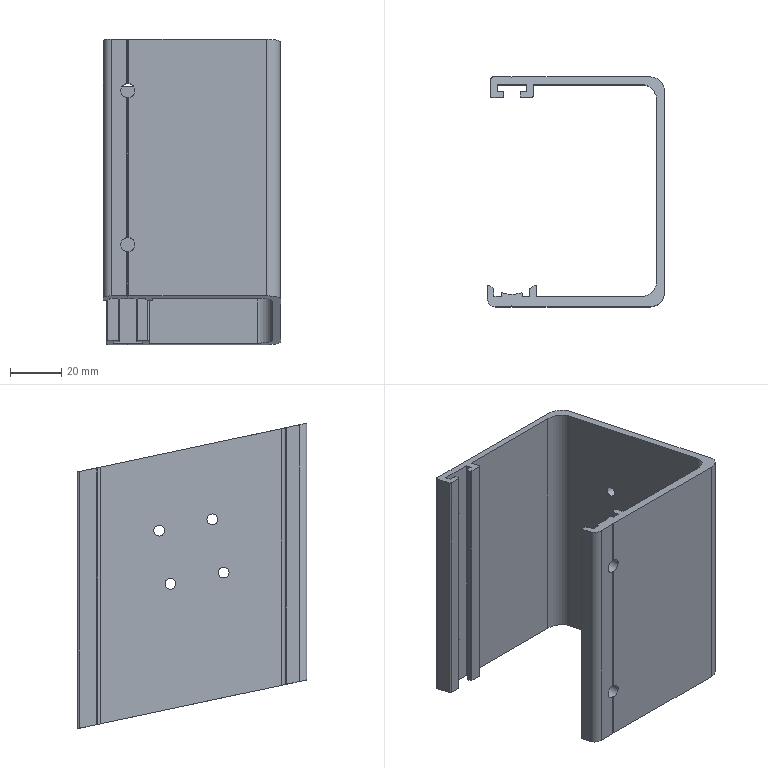Part | STEP file | 31E-01018XJ10 | 1 solid | 78 faces | box 69 x 89.5 x 119.024 mm | volume 78639 mm3 | plane 41 | cylinder 37 | commonest cylinder face diameters 1 x10 4.2 x8 3.2 x4 5.5 x4 25.4 x3 0.4 x2